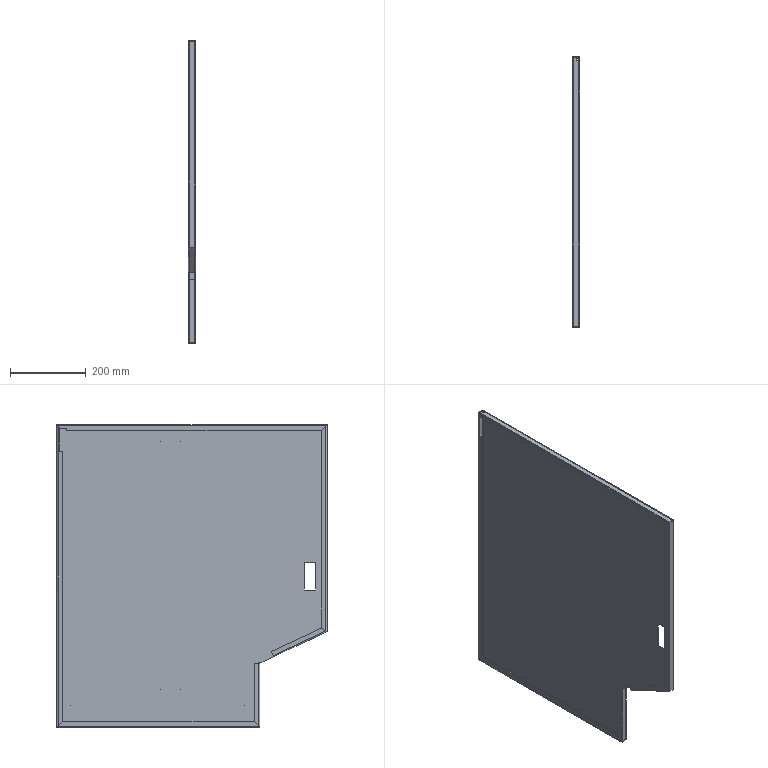Part | NX | features solid 2 | 1 solid | 190 faces | box 20 x 713.5 x 799 mm | volume 924165 mm3 | plane 105 | cylinder 46 | spline 39 | commonest cylinder face diameters 6 x16 1 x12 3 x12 7 x4 4 x2